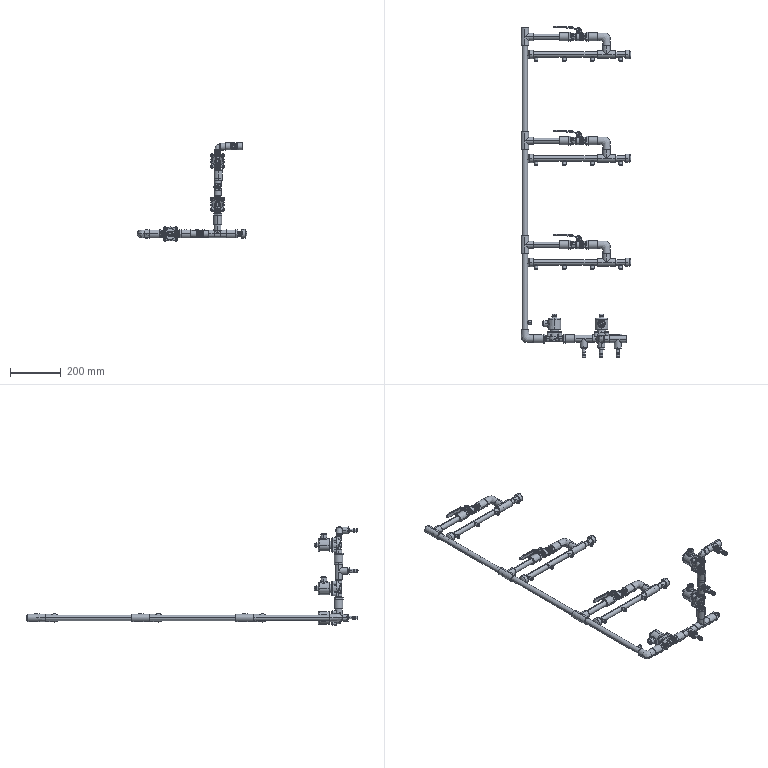Part | SolidWorks | 114 solids | 5138 faces | volume 2028858 mm3 | cylinder 1442 | plane 1244 | cone 1033 | spline 1022 | torus 241 | sphere 156 | commonest cylinder face diameters 0.635 x186 19.583 x120 18.5 x111 13.868 x107 7 x81 10 x74